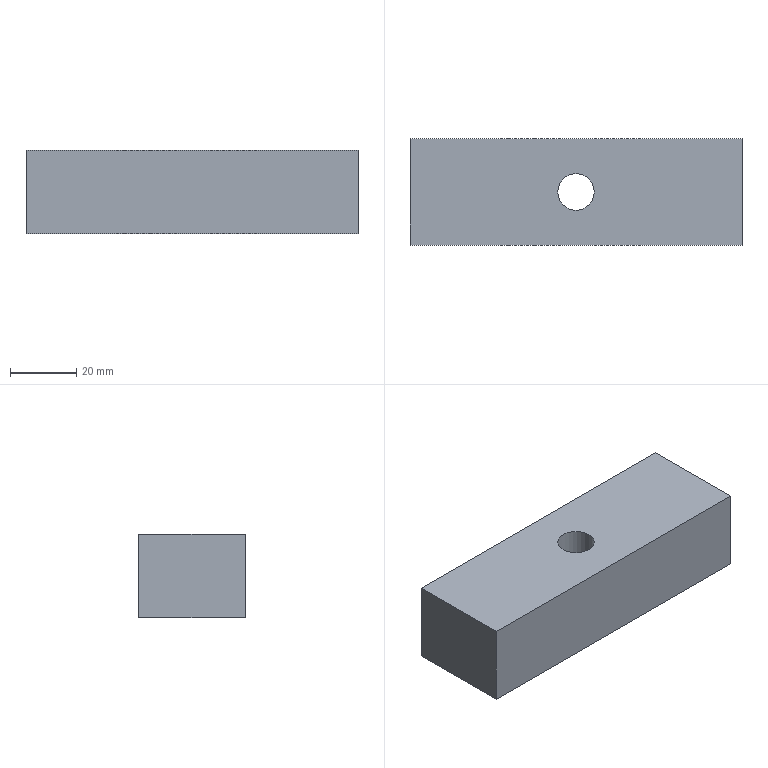Part | NX | features solid 2 | 1 solid | 9 faces | box 100 x 32 x 25 mm | volume 75711 mm3 | plane 7 | cylinder 2 | commonest cylinder face diameters 11 x1 18 x1
STEP:
#1=CARTESIAN_POINT('',(-1005.,-419.,143.));
#2=VERTEX_POINT('',#1);
#3=CARTESIAN_POINT('',(-1005.,-419.,118.));
#4=VERTEX_POINT('',#3);
#5=CARTESIAN_POINT('',(-1005.,-419.,143.));
#6=DIRECTION('',(0.,0.,-1.));
#7=VECTOR('',#6,1000.);
#8=LINE('',#5,#7);
#9=EDGE_CURVE('',#2,#4,#8,.T.);
#10=ORIENTED_EDGE('',*,*,#9,.T.);
#11=CARTESIAN_POINT('',(-1105.,-419.,118.));
#12=VERTEX_POINT('',#11);
#13=CARTESIAN_POINT('',(-1110.,-419.,118.));
#14=DIRECTION('',(-1.,0.,0.));
#15=VECTOR('',#14,1000.);
#16=LINE('',#13,#15);
#17=EDGE_CURVE('',#12,#4,#16,.F.);
#18=ORIENTED_EDGE('',*,*,#17,.F.);
#19=CARTESIAN_POINT('',(-1105.,-419.,143.));
#20=VERTEX_POINT('',#19);
#21=CARTESIAN_POINT('',(-1105.,-419.,143.));
#22=DIRECTION('',(0.,0.,-1.));
#23=VECTOR('',#22,1000.);
#24=LINE('',#21,#23);
#25=EDGE_CURVE('',#20,#12,#24,.T.);
#26=ORIENTED_EDGE('',*,*,#25,.F.);
#27=CARTESIAN_POINT('',(-1110.,-419.,143.));
#28=DIRECTION('',(1.,0.,0.));
#29=VECTOR('',#28,1000.);
#30=LINE('',#27,#29);
#31=EDGE_CURVE('',#20,#2,#30,.T.);
#32=ORIENTED_EDGE('',*,*,#31,.T.);
#33=EDGE_LOOP('',(#10,#18,#26,#32));
#34=FACE_BOUND('',#33,.T.);
#35=CARTESIAN_POINT('',(-1110.,-419.,143.));
#36=DIRECTION('',(0.,1.,0.));
#37=DIRECTION('',(1.,0.,0.));
#38=AXIS2_PLACEMENT_3D('',#35,#36,#37);
#39=PLANE('',#38);
#40=ADVANCED_FACE('',(#34),#39,.T.);
#41=ORIENTED_EDGE('',*,*,#25,.T.);
#42=CARTESIAN_POINT('',(-1105.,-451.,118.));
#43=VERTEX_POINT('',#42);
#44=CARTESIAN_POINT('',(-1105.,-419.,118.));
#45=DIRECTION('',(0.,1.,0.));
#46=VECTOR('',#45,1000.);
#47=LINE('',#44,#46);
#48=EDGE_CURVE('',#12,#43,#47,.F.);
#49=ORIENTED_EDGE('',*,*,#48,.T.);
#50=CARTESIAN_POINT('',(-1105.,-451.,143.));
#51=VERTEX_POINT('',#50);
#52=CARTESIAN_POINT('',(-1105.,-451.,143.));
#53=DIRECTION('',(0.,0.,-1.));
#54=VECTOR('',#53,1000.);
#55=LINE('',#52,#54);
#56=EDGE_CURVE('',#51,#43,#55,.T.);
#57=ORIENTED_EDGE('',*,*,#56,.F.);
#58=CARTESIAN_POINT('',(-1105.,-419.,143.));
#59=DIRECTION('',(0.,-1.,0.));
#60=VECTOR('',#59,1000.);
#61=LINE('',#58,#60);
#62=EDGE_CURVE('',#20,#51,#61,.T.);
#63=ORIENTED_EDGE('',*,*,#62,.F.);
#64=EDGE_LOOP('',(#41,#49,#57,#63));
#65=FACE_BOUND('',#64,.T.);
#66=CARTESIAN_POINT('',(-1105.,-419.,143.));
#67=DIRECTION('',(1.,0.,0.));
#68=DIRECTION('',(0.,-1.,0.));
#69=AXIS2_PLACEMENT_3D('',#66,#67,#68);
#70=PLANE('',#69);
#71=ADVANCED_FACE('',(#65),#70,.F.);
#72=ORIENTED_EDGE('',*,*,#56,.T.);
#73=CARTESIAN_POINT('',(-1005.,-451.,118.));
#74=VERTEX_POINT('',#73);
#75=CARTESIAN_POINT('',(-1110.,-451.,118.));
#76=DIRECTION('',(-1.,0.,0.));
#77=VECTOR('',#76,1000.);
#78=LINE('',#75,#77);
#79=EDGE_CURVE('',#43,#74,#78,.F.);
#80=ORIENTED_EDGE('',*,*,#79,.T.);
#81=CARTESIAN_POINT('',(-1005.,-451.,143.));
#82=VERTEX_POINT('',#81);
#83=CARTESIAN_POINT('',(-1005.,-451.,143.));
#84=DIRECTION('',(0.,0.,-1.));
#85=VECTOR('',#84,1000.);
#86=LINE('',#83,#85);
#87=EDGE_CURVE('',#82,#74,#86,.T.);
#88=ORIENTED_EDGE('',*,*,#87,.F.);
#89=CARTESIAN_POINT('',(-1110.,-451.,143.));
#90=DIRECTION('',(1.,0.,0.));
#91=VECTOR('',#90,1000.);
#92=LINE('',#89,#91);
#93=EDGE_CURVE('',#51,#82,#92,.T.);
#94=ORIENTED_EDGE('',*,*,#93,.F.);
#95=EDGE_LOOP('',(#72,#80,#88,#94));
#96=FACE_BOUND('',#95,.T.);
#97=CARTESIAN_POINT('',(-1110.,-451.,143.));
#98=DIRECTION('',(0.,1.,0.));
#99=DIRECTION('',(1.,0.,0.));
#100=AXIS2_PLACEMENT_3D('',#97,#98,#99);
#101=PLANE('',#100);
#102=ADVANCED_FACE('',(#96),#101,.F.);
#103=CARTESIAN_POINT('',(-1005.,-419.,143.));
#104=DIRECTION('',(0.,-1.,0.));
#105=VECTOR('',#104,1000.);
#106=LINE('',#103,#105);
#107=EDGE_CURVE('',#2,#82,#106,.T.);
#108=ORIENTED_EDGE('',*,*,#107,.T.);
#109=ORIENTED_EDGE('',*,*,#87,.T.);
#110=CARTESIAN_POINT('',(-1005.,-419.,118.));
#111=DIRECTION('',(0.,1.,0.));
#112=VECTOR('',#111,1000.);
#113=LINE('',#110,#112);
#114=EDGE_CURVE('',#4,#74,#113,.F.);
#115=ORIENTED_EDGE('',*,*,#114,.F.);
#116=ORIENTED_EDGE('',*,*,#9,.F.);
#117=EDGE_LOOP('',(#108,#109,#115,#116));
#118=FACE_BOUND('',#117,.T.);
#119=CARTESIAN_POINT('',(-1005.,-419.,143.));
#120=DIRECTION('',(1.,0.,0.));
#121=DIRECTION('',(0.,-1.,0.));
#122=AXIS2_PLACEMENT_3D('',#119,#120,#121);
#123=PLANE('',#122);
#124=ADVANCED_FACE('',(#118),#123,.T.);
#125=CARTESIAN_POINT('',(-1064.,-435.,118.));
#126=VERTEX_POINT('',#125);
#127=CARTESIAN_POINT('',(-1055.,-435.,118.));
#128=DIRECTION('',(0.,0.,-1.));
#129=DIRECTION('',(-1.,0.,0.));
#130=AXIS2_PLACEMENT_3D('',#127,#128,#129);
#131=CIRCLE('',#130,9.);
#132=EDGE_CURVE('',#126,#126,#131,.T.);
#133=ORIENTED_EDGE('',*,*,#132,.F.);
#134=EDGE_LOOP('',(#133));
#135=FACE_BOUND('',#134,.T.);
#136=ORIENTED_EDGE('',*,*,#79,.F.);
#137=ORIENTED_EDGE('',*,*,#48,.F.);
#138=ORIENTED_EDGE('',*,*,#17,.T.);
#139=ORIENTED_EDGE('',*,*,#114,.T.);
#140=EDGE_LOOP('',(#136,#137,#138,#139));
#141=FACE_BOUND('',#140,.T.);
#142=CARTESIAN_POINT('',(-1110.,-419.,118.));
#143=DIRECTION('',(0.,0.,1.));
#144=DIRECTION('',(-1.,0.,0.));
#145=AXIS2_PLACEMENT_3D('',#142,#143,#144);
#146=PLANE('',#145);
#147=ADVANCED_FACE('',(#135,#141),#146,.F.);
#148=CARTESIAN_POINT('',(-1060.5,-435.,143.));
#149=VERTEX_POINT('',#148);
#150=CARTESIAN_POINT('',(-1055.,-435.,143.));
#151=DIRECTION('',(0.,0.,-1.));
#152=DIRECTION('',(-1.,0.,0.));
#153=AXIS2_PLACEMENT_3D('',#150,#151,#152);
#154=CIRCLE('',#153,5.5);
#155=EDGE_CURVE('',#149,#149,#154,.T.);
#156=ORIENTED_EDGE('',*,*,#155,.T.);
#157=EDGE_LOOP('',(#156));
#158=FACE_BOUND('',#157,.T.);
#159=ORIENTED_EDGE('',*,*,#93,.T.);
#160=ORIENTED_EDGE('',*,*,#107,.F.);
#161=ORIENTED_EDGE('',*,*,#31,.F.);
#162=ORIENTED_EDGE('',*,*,#62,.T.);
#163=EDGE_LOOP('',(#159,#160,#161,#162));
#164=FACE_BOUND('',#163,.T.);
#165=CARTESIAN_POINT('',(-1110.,-419.,143.));
#166=DIRECTION('',(0.,0.,1.));
#167=DIRECTION('',(-1.,0.,0.));
#168=AXIS2_PLACEMENT_3D('',#165,#166,#167);
#169=PLANE('',#168);
#170=ADVANCED_FACE('',(#158,#164),#169,.T.);
#171=ORIENTED_EDGE('',*,*,#155,.F.);
#172=EDGE_LOOP('',(#171));
#173=FACE_BOUND('',#172,.T.);
#174=CARTESIAN_POINT('',(-1060.5,-435.,130.));
#175=VERTEX_POINT('',#174);
#176=CARTESIAN_POINT('',(-1055.,-435.,130.));
#177=DIRECTION('',(0.,0.,-1.));
#178=DIRECTION('',(-1.,0.,0.));
#179=AXIS2_PLACEMENT_3D('',#176,#177,#178);
#180=CIRCLE('',#179,5.5);
#181=EDGE_CURVE('',#175,#175,#180,.T.);
#182=ORIENTED_EDGE('',*,*,#181,.T.);
#183=EDGE_LOOP('',(#182));
#184=FACE_BOUND('',#183,.T.);
#185=CARTESIAN_POINT('',(-1055.,-435.,168.));
#186=DIRECTION('',(0.,0.,1.));
#187=DIRECTION('',(-1.,0.,0.));
#188=AXIS2_PLACEMENT_3D('',#185,#186,#187);
#189=CYLINDRICAL_SURFACE('',#188,5.5);
#190=ADVANCED_FACE('',(#173,#184),#189,.F.);
#191=ORIENTED_EDGE('',*,*,#181,.F.);
#192=EDGE_LOOP('',(#191));
#193=FACE_BOUND('',#192,.T.);
#194=CARTESIAN_POINT('',(-1064.,-435.,130.));
#195=VERTEX_POINT('',#194);
#196=CARTESIAN_POINT('',(-1055.,-435.,130.));
#197=DIRECTION('',(0.,0.,-1.));
#198=DIRECTION('',(-1.,0.,0.));
#199=AXIS2_PLACEMENT_3D('',#196,#197,#198);
#200=CIRCLE('',#199,9.);
#201=EDGE_CURVE('',#195,#195,#200,.T.);
#202=ORIENTED_EDGE('',*,*,#201,.T.);
#203=EDGE_LOOP('',(#202));
#204=FACE_BOUND('',#203,.T.);
#205=CARTESIAN_POINT('',(-1055.,-435.,130.));
#206=DIRECTION('',(0.,0.,1.));
#207=DIRECTION('',(-1.,0.,0.));
#208=AXIS2_PLACEMENT_3D('',#205,#206,#207);
#209=PLANE('',#208);
#210=ADVANCED_FACE('',(#193,#204),#209,.F.);
#211=ORIENTED_EDGE('',*,*,#201,.F.);
#212=EDGE_LOOP('',(#211));
#213=FACE_BOUND('',#212,.T.);
#214=ORIENTED_EDGE('',*,*,#132,.T.);
#215=EDGE_LOOP('',(#214));
#216=FACE_BOUND('',#215,.T.);
#217=CARTESIAN_POINT('',(-1055.,-435.,118.));
#218=DIRECTION('',(0.,0.,1.));
#219=DIRECTION('',(-1.,0.,0.));
#220=AXIS2_PLACEMENT_3D('',#217,#218,#219);
#221=CYLINDRICAL_SURFACE('',#220,9.);
#222=ADVANCED_FACE('',(#213,#216),#221,.F.);
#223=CLOSED_SHELL('',(#40,#71,#102,#124,#147,#170,#190,#210,#222));
#224=MANIFOLD_SOLID_BREP('',#223);
#225=(LENGTH_UNIT()NAMED_UNIT(*)SI_UNIT(.MILLI.,.METRE.));
#226=UNCERTAINTY_MEASURE_WITH_UNIT(LENGTH_MEASURE(0.00001),#225,'','');
#227=(NAMED_UNIT(*)PLANE_ANGLE_UNIT()SI_UNIT($,.RADIAN.));
#228=(NAMED_UNIT(*)SI_UNIT($,.STERADIAN.)SOLID_ANGLE_UNIT());
#229=(GEOMETRIC_REPRESENTATION_CONTEXT(3)GLOBAL_UNCERTAINTY_ASSIGNED_CONTEXT((#226))GLOBAL_UNIT_ASSIGNED_CONTEXT((#225,#227,#228))REPRESENTATION_CONTEXT('',''));
#230=ADVANCED_BREP_SHAPE_REPRESENTATION('',(#224),#229);